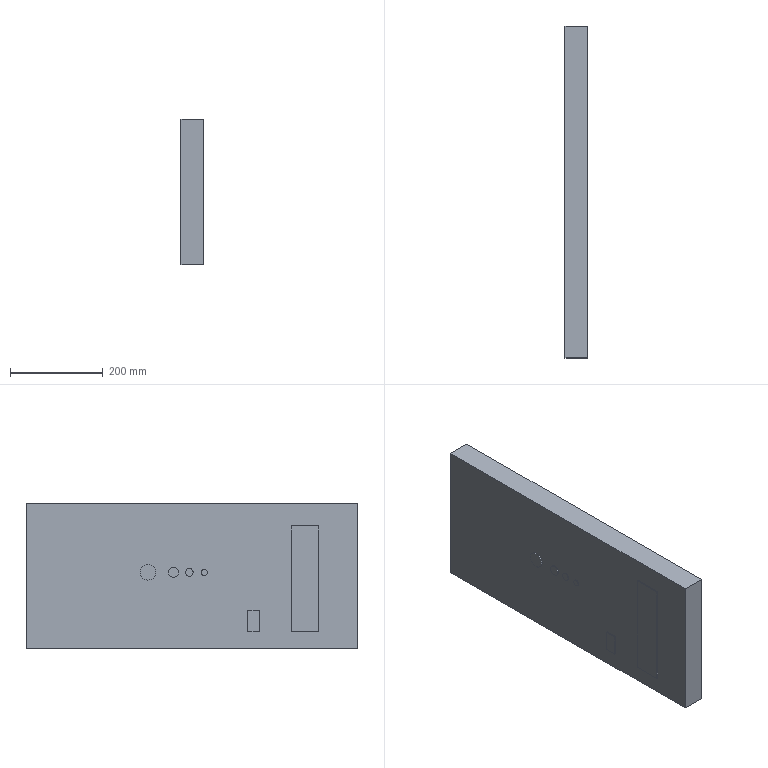Part | STEP file | 1 solid | 28 faces | box 51.504 x 714.237 x 313.918 mm | volume 11131790 mm3 | plane 20 | cylinder 8 | commonest cylinder face diameters 13.163 x2 16.558 x2 21.583 x2 33.527 x2